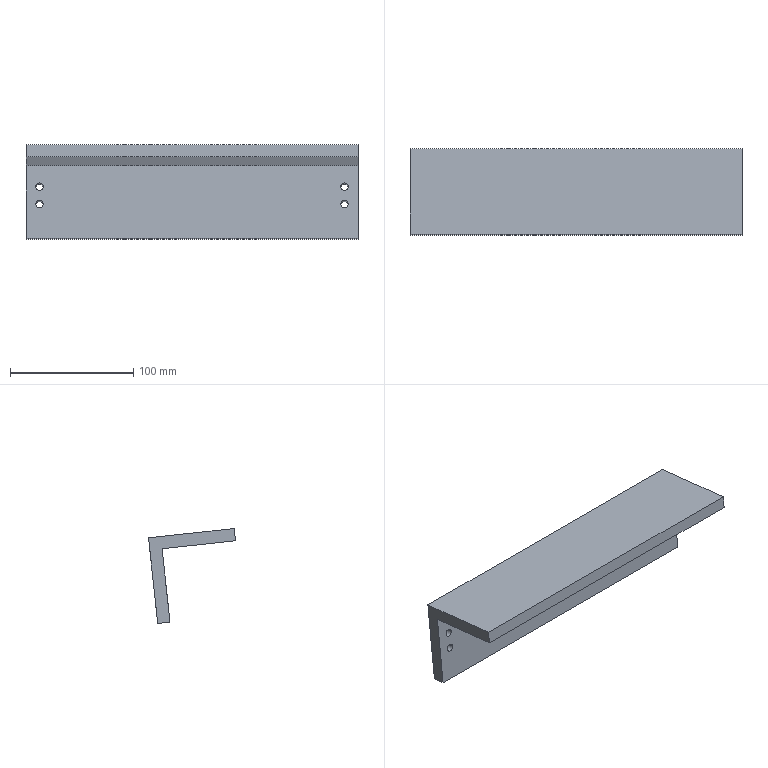Part | STEP file | Fillet 1-6 | 1 solid | 17 faces | box 269.706 x 70.669 x 77.109 mm | volume 349545 mm3 | cylinder 9 | plane 8 | commonest cylinder face diameters 6 x8 2 x1
STEP:
#1=CARTESIAN_POINT('',(40.034,-1255.734,3546.775));
#2=VERTEX_POINT('',#1);
#3=CARTESIAN_POINT('',(46.034,-1255.734,3546.775));
#4=VERTEX_POINT('',#3);
#5=CARTESIAN_POINT('',(43.034,-1255.734,3546.775));
#6=DIRECTION('',(0.,0.9942,-0.1073));
#7=DIRECTION('',(-1.,0.,0.));
#8=AXIS2_PLACEMENT_3D('',#5,#6,#7);
#9=CIRCLE('',#8,3.);
#10=EDGE_CURVE('',#2,#4,#9,.T.);
#11=ORIENTED_EDGE('',*,*,#10,.F.);
#12=CARTESIAN_POINT('',(40.034,-1245.792,3545.702));
#13=VERTEX_POINT('',#12);
#14=CARTESIAN_POINT('',(40.034,-1255.734,3546.775));
#15=DIRECTION('',(0.,0.9942,-0.1073));
#16=VECTOR('',#15,1000.);
#17=LINE('',#14,#16);
#18=EDGE_CURVE('',#2,#13,#17,.T.);
#19=ORIENTED_EDGE('',*,*,#18,.T.);
#20=CARTESIAN_POINT('',(46.034,-1245.792,3545.702));
#21=VERTEX_POINT('',#20);
#22=CARTESIAN_POINT('',(43.034,-1245.792,3545.702));
#23=DIRECTION('',(0.,0.9942,-0.1073));
#24=DIRECTION('',(-1.,0.,0.));
#25=AXIS2_PLACEMENT_3D('',#22,#23,#24);
#26=CIRCLE('',#25,3.);
#27=EDGE_CURVE('',#13,#21,#26,.T.);
#28=ORIENTED_EDGE('',*,*,#27,.T.);
#29=CARTESIAN_POINT('',(46.034,-1255.734,3546.775));
#30=DIRECTION('',(0.,0.9942,-0.1073));
#31=VECTOR('',#30,1000.);
#32=LINE('',#29,#31);
#33=EDGE_CURVE('',#4,#21,#32,.T.);
#34=ORIENTED_EDGE('',*,*,#33,.F.);
#35=EDGE_LOOP('',(#11,#19,#28,#34));
#36=FACE_OUTER_BOUND('',#35,.T.);
#37=CARTESIAN_POINT('',(43.034,-1255.734,3546.775));
#38=DIRECTION('',(0.,0.9942,-0.1073));
#39=DIRECTION('',(-1.,0.,0.));
#40=AXIS2_PLACEMENT_3D('',#37,#38,#39);
#41=CYLINDRICAL_SURFACE('',#40,3.);
#42=ADVANCED_FACE('',(#36),#41,.F.);
#43=CARTESIAN_POINT('',(287.74,-1254.205,3560.936));
#44=VERTEX_POINT('',#43);
#45=CARTESIAN_POINT('',(293.74,-1254.205,3560.936));
#46=VERTEX_POINT('',#45);
#47=CARTESIAN_POINT('',(290.74,-1254.205,3560.936));
#48=DIRECTION('',(0.,0.9942,-0.1073));
#49=DIRECTION('',(-1.,0.,0.));
#50=AXIS2_PLACEMENT_3D('',#47,#48,#49);
#51=CIRCLE('',#50,3.);
#52=EDGE_CURVE('',#44,#46,#51,.T.);
#53=ORIENTED_EDGE('',*,*,#52,.F.);
#54=CARTESIAN_POINT('',(287.74,-1244.263,3559.863));
#55=VERTEX_POINT('',#54);
#56=CARTESIAN_POINT('',(287.74,-1254.205,3560.936));
#57=DIRECTION('',(0.,0.9942,-0.1073));
#58=VECTOR('',#57,1000.);
#59=LINE('',#56,#58);
#60=EDGE_CURVE('',#44,#55,#59,.T.);
#61=ORIENTED_EDGE('',*,*,#60,.T.);
#62=CARTESIAN_POINT('',(293.74,-1244.263,3559.863));
#63=VERTEX_POINT('',#62);
#64=CARTESIAN_POINT('',(290.74,-1244.263,3559.863));
#65=DIRECTION('',(0.,0.9942,-0.1073));
#66=DIRECTION('',(-1.,0.,0.));
#67=AXIS2_PLACEMENT_3D('',#64,#65,#66);
#68=CIRCLE('',#67,3.);
#69=EDGE_CURVE('',#55,#63,#68,.T.);
#70=ORIENTED_EDGE('',*,*,#69,.T.);
#71=CARTESIAN_POINT('',(293.74,-1254.205,3560.936));
#72=DIRECTION('',(0.,0.9942,-0.1073));
#73=VECTOR('',#72,1000.);
#74=LINE('',#71,#73);
#75=EDGE_CURVE('',#46,#63,#74,.T.);
#76=ORIENTED_EDGE('',*,*,#75,.F.);
#77=EDGE_LOOP('',(#53,#61,#70,#76));
#78=FACE_OUTER_BOUND('',#77,.T.);
#79=CARTESIAN_POINT('',(290.74,-1254.205,3560.936));
#80=DIRECTION('',(0.,0.9942,-0.1073));
#81=DIRECTION('',(-1.,0.,0.));
#82=AXIS2_PLACEMENT_3D('',#79,#80,#81);
#83=CYLINDRICAL_SURFACE('',#82,3.);
#84=ADVANCED_FACE('',(#78),#83,.F.);
#85=CARTESIAN_POINT('',(287.74,-1255.734,3546.775));
#86=VERTEX_POINT('',#85);
#87=CARTESIAN_POINT('',(293.74,-1255.734,3546.775));
#88=VERTEX_POINT('',#87);
#89=CARTESIAN_POINT('',(290.74,-1255.734,3546.775));
#90=DIRECTION('',(0.,0.9942,-0.1073));
#91=DIRECTION('',(1.,0.,0.));
#92=AXIS2_PLACEMENT_3D('',#89,#90,#91);
#93=CIRCLE('',#92,3.);
#94=EDGE_CURVE('',#86,#88,#93,.T.);
#95=ORIENTED_EDGE('',*,*,#94,.F.);
#96=CARTESIAN_POINT('',(287.74,-1245.792,3545.702));
#97=VERTEX_POINT('',#96);
#98=CARTESIAN_POINT('',(287.74,-1255.734,3546.775));
#99=DIRECTION('',(0.,0.9942,-0.1073));
#100=VECTOR('',#99,1000.);
#101=LINE('',#98,#100);
#102=EDGE_CURVE('',#86,#97,#101,.T.);
#103=ORIENTED_EDGE('',*,*,#102,.T.);
#104=CARTESIAN_POINT('',(293.74,-1245.792,3545.702));
#105=VERTEX_POINT('',#104);
#106=CARTESIAN_POINT('',(290.74,-1245.792,3545.702));
#107=DIRECTION('',(0.,0.9942,-0.1073));
#108=DIRECTION('',(1.,0.,0.));
#109=AXIS2_PLACEMENT_3D('',#106,#107,#108);
#110=CIRCLE('',#109,3.);
#111=EDGE_CURVE('',#97,#105,#110,.T.);
#112=ORIENTED_EDGE('',*,*,#111,.T.);
#113=CARTESIAN_POINT('',(293.74,-1255.734,3546.775));
#114=DIRECTION('',(0.,0.9942,-0.1073));
#115=VECTOR('',#114,1000.);
#116=LINE('',#113,#115);
#117=EDGE_CURVE('',#88,#105,#116,.T.);
#118=ORIENTED_EDGE('',*,*,#117,.F.);
#119=EDGE_LOOP('',(#95,#103,#112,#118));
#120=FACE_OUTER_BOUND('',#119,.T.);
#121=CARTESIAN_POINT('',(290.74,-1255.734,3546.775));
#122=DIRECTION('',(0.,0.9942,-0.1073));
#123=DIRECTION('',(-1.,0.,0.));
#124=AXIS2_PLACEMENT_3D('',#121,#122,#123);
#125=CYLINDRICAL_SURFACE('',#124,3.);
#126=ADVANCED_FACE('',(#120),#125,.F.);
#127=CARTESIAN_POINT('',(40.034,-1254.205,3560.936));
#128=VERTEX_POINT('',#127);
#129=CARTESIAN_POINT('',(46.034,-1254.205,3560.936));
#130=VERTEX_POINT('',#129);
#131=CARTESIAN_POINT('',(43.034,-1254.205,3560.936));
#132=DIRECTION('',(0.,0.9942,-0.1073));
#133=DIRECTION('',(1.,0.,0.));
#134=AXIS2_PLACEMENT_3D('',#131,#132,#133);
#135=CIRCLE('',#134,3.);
#136=EDGE_CURVE('',#128,#130,#135,.T.);
#137=ORIENTED_EDGE('',*,*,#136,.F.);
#138=CARTESIAN_POINT('',(40.034,-1244.263,3559.863));
#139=VERTEX_POINT('',#138);
#140=CARTESIAN_POINT('',(40.034,-1254.205,3560.936));
#141=DIRECTION('',(0.,0.9942,-0.1073));
#142=VECTOR('',#141,1000.);
#143=LINE('',#140,#142);
#144=EDGE_CURVE('',#128,#139,#143,.T.);
#145=ORIENTED_EDGE('',*,*,#144,.T.);
#146=CARTESIAN_POINT('',(46.034,-1244.263,3559.863));
#147=VERTEX_POINT('',#146);
#148=CARTESIAN_POINT('',(43.034,-1244.263,3559.863));
#149=DIRECTION('',(0.,0.9942,-0.1073));
#150=DIRECTION('',(1.,0.,0.));
#151=AXIS2_PLACEMENT_3D('',#148,#149,#150);
#152=CIRCLE('',#151,3.);
#153=EDGE_CURVE('',#139,#147,#152,.T.);
#154=ORIENTED_EDGE('',*,*,#153,.T.);
#155=CARTESIAN_POINT('',(46.034,-1254.205,3560.936));
#156=DIRECTION('',(0.,0.9942,-0.1073));
#157=VECTOR('',#156,1000.);
#158=LINE('',#155,#157);
#159=EDGE_CURVE('',#130,#147,#158,.T.);
#160=ORIENTED_EDGE('',*,*,#159,.F.);
#161=EDGE_LOOP('',(#137,#145,#154,#160));
#162=FACE_OUTER_BOUND('',#161,.T.);
#163=CARTESIAN_POINT('',(43.034,-1254.205,3560.936));
#164=DIRECTION('',(0.,0.9942,-0.1073));
#165=DIRECTION('',(-1.,0.,0.));
#166=AXIS2_PLACEMENT_3D('',#163,#164,#165);
#167=CYLINDRICAL_SURFACE('',#166,3.);
#168=ADVANCED_FACE('',(#162),#167,.F.);
#169=CARTESIAN_POINT('',(43.034,-1255.734,3546.775));
#170=DIRECTION('',(0.,0.9942,-0.1073));
#171=DIRECTION('',(-1.,0.,0.));
#172=AXIS2_PLACEMENT_3D('',#169,#170,#171);
#173=CIRCLE('',#172,3.);
#174=EDGE_CURVE('',#4,#2,#173,.T.);
#175=ORIENTED_EDGE('',*,*,#174,.T.);
#176=ORIENTED_EDGE('',*,*,#10,.T.);
#177=EDGE_LOOP('',(#175,#176));
#178=FACE_BOUND('',#177,.T.);
#179=CARTESIAN_POINT('',(290.74,-1254.205,3560.936));
#180=DIRECTION('',(0.,0.9942,-0.1073));
#181=DIRECTION('',(-1.,0.,0.));
#182=AXIS2_PLACEMENT_3D('',#179,#180,#181);
#183=CIRCLE('',#182,3.);
#184=EDGE_CURVE('',#46,#44,#183,.T.);
#185=ORIENTED_EDGE('',*,*,#184,.T.);
#186=ORIENTED_EDGE('',*,*,#52,.T.);
#187=EDGE_LOOP('',(#185,#186));
#188=FACE_BOUND('',#187,.T.);
#189=CARTESIAN_POINT('',(290.74,-1255.734,3546.775));
#190=DIRECTION('',(0.,0.9942,-0.1073));
#191=DIRECTION('',(1.,0.,0.));
#192=AXIS2_PLACEMENT_3D('',#189,#190,#191);
#193=CIRCLE('',#192,3.);
#194=EDGE_CURVE('',#88,#86,#193,.T.);
#195=ORIENTED_EDGE('',*,*,#194,.T.);
#196=ORIENTED_EDGE('',*,*,#94,.T.);
#197=EDGE_LOOP('',(#195,#196));
#198=FACE_BOUND('',#197,.T.);
#199=CARTESIAN_POINT('',(43.034,-1254.205,3560.936));
#200=DIRECTION('',(0.,0.9942,-0.1073));
#201=DIRECTION('',(1.,0.,0.));
#202=AXIS2_PLACEMENT_3D('',#199,#200,#201);
#203=CIRCLE('',#202,3.);
#204=EDGE_CURVE('',#130,#128,#203,.T.);
#205=ORIENTED_EDGE('',*,*,#204,.T.);
#206=ORIENTED_EDGE('',*,*,#136,.T.);
#207=EDGE_LOOP('',(#205,#206));
#208=FACE_BOUND('',#207,.T.);
#209=CARTESIAN_POINT('',(301.74,-1252.394,3577.717));
#210=VERTEX_POINT('',#209);
#211=CARTESIAN_POINT('',(301.74,-1258.727,3519.058));
#212=VERTEX_POINT('',#211);
#213=CARTESIAN_POINT('',(301.74,-1251.213,3588.654));
#214=DIRECTION('',(0.,-0.1073,-0.9942));
#215=VECTOR('',#214,1000.);
#216=LINE('',#213,#215);
#217=EDGE_CURVE('',#210,#212,#216,.T.);
#218=ORIENTED_EDGE('',*,*,#217,.F.);
#219=CARTESIAN_POINT('',(32.034,-1252.394,3577.717));
#220=VERTEX_POINT('',#219);
#221=CARTESIAN_POINT('',(166.887,-1252.394,3577.717));
#222=DIRECTION('',(-1.,0.,0.));
#223=VECTOR('',#222,1000.);
#224=LINE('',#221,#223);
#225=EDGE_CURVE('',#210,#220,#224,.T.);
#226=ORIENTED_EDGE('',*,*,#225,.T.);
#227=CARTESIAN_POINT('',(32.034,-1258.727,3519.058));
#228=VERTEX_POINT('',#227);
#229=CARTESIAN_POINT('',(32.034,-1251.213,3588.654));
#230=DIRECTION('',(0.,0.1073,0.9942));
#231=VECTOR('',#230,1000.);
#232=LINE('',#229,#231);
#233=EDGE_CURVE('',#228,#220,#232,.T.);
#234=ORIENTED_EDGE('',*,*,#233,.F.);
#235=CARTESIAN_POINT('',(32.034,-1258.727,3519.058));
#236=DIRECTION('',(-1.,0.,0.));
#237=VECTOR('',#236,1000.);
#238=LINE('',#235,#237);
#239=EDGE_CURVE('',#212,#228,#238,.T.);
#240=ORIENTED_EDGE('',*,*,#239,.F.);
#241=EDGE_LOOP('',(#218,#226,#234,#240));
#242=FACE_OUTER_BOUND('',#241,.T.);
#243=CARTESIAN_POINT('',(166.887,-1254.97,3553.856));
#244=DIRECTION('',(0.,-0.9942,0.1073));
#245=DIRECTION('',(1.,0.,0.));
#246=AXIS2_PLACEMENT_3D('',#243,#244,#245);
#247=PLANE('',#246);
#248=ADVANCED_FACE('',(#178,#188,#198,#208,#242),#247,.T.);
#249=CARTESIAN_POINT('',(301.74,-1241.271,3587.58));
#250=VERTEX_POINT('',#249);
#251=CARTESIAN_POINT('',(301.74,-1310.866,3595.094));
#252=VERTEX_POINT('',#251);
#253=CARTESIAN_POINT('',(301.74,-1241.271,3587.58));
#254=DIRECTION('',(0.,-0.9942,0.1073));
#255=VECTOR('',#254,1000.);
#256=LINE('',#253,#255);
#257=EDGE_CURVE('',#250,#252,#256,.T.);
#258=ORIENTED_EDGE('',*,*,#257,.T.);
#259=CARTESIAN_POINT('',(301.74,-1311.94,3585.152));
#260=VERTEX_POINT('',#259);
#261=CARTESIAN_POINT('',(301.74,-1311.94,3585.152));
#262=DIRECTION('',(0.,0.1073,0.9942));
#263=VECTOR('',#262,1000.);
#264=LINE('',#261,#263);
#265=EDGE_CURVE('',#260,#252,#264,.T.);
#266=ORIENTED_EDGE('',*,*,#265,.F.);
#267=CARTESIAN_POINT('',(301.74,-1253.281,3578.819));
#268=VERTEX_POINT('',#267);
#269=CARTESIAN_POINT('',(301.74,-1311.94,3585.152));
#270=DIRECTION('',(0.,0.9942,-0.1073));
#271=VECTOR('',#270,1000.);
#272=LINE('',#269,#271);
#273=EDGE_CURVE('',#260,#268,#272,.T.);
#274=ORIENTED_EDGE('',*,*,#273,.T.);
#275=CARTESIAN_POINT('',(301.74,-1253.388,3577.825));
#276=DIRECTION('',(-1.,0.,0.));
#277=DIRECTION('',(0.,0.9942,-0.1073));
#278=AXIS2_PLACEMENT_3D('',#275,#276,#277);
#279=CIRCLE('',#278,1.);
#280=EDGE_CURVE('',#268,#210,#279,.T.);
#281=ORIENTED_EDGE('',*,*,#280,.T.);
#282=ORIENTED_EDGE('',*,*,#217,.T.);
#283=CARTESIAN_POINT('',(301.74,-1248.785,3517.985));
#284=VERTEX_POINT('',#283);
#285=CARTESIAN_POINT('',(301.74,-1248.785,3517.985));
#286=DIRECTION('',(0.,-0.9942,0.1073));
#287=VECTOR('',#286,1000.);
#288=LINE('',#285,#287);
#289=EDGE_CURVE('',#284,#212,#288,.T.);
#290=ORIENTED_EDGE('',*,*,#289,.F.);
#291=CARTESIAN_POINT('',(301.74,-1241.271,3587.58));
#292=DIRECTION('',(0.,-0.1073,-0.9942));
#293=VECTOR('',#292,1000.);
#294=LINE('',#291,#293);
#295=EDGE_CURVE('',#250,#284,#294,.T.);
#296=ORIENTED_EDGE('',*,*,#295,.F.);
#297=EDGE_LOOP('',(#258,#266,#274,#281,#282,#290,#296));
#298=FACE_OUTER_BOUND('',#297,.T.);
#299=CARTESIAN_POINT('',(301.74,-1241.271,3587.58));
#300=DIRECTION('',(-1.,0.,0.));
#301=DIRECTION('',(0.,-0.9942,0.1073));
#302=AXIS2_PLACEMENT_3D('',#299,#300,#301);
#303=PLANE('',#302);
#304=ADVANCED_FACE('',(#298),#303,.F.);
#305=ORIENTED_EDGE('',*,*,#239,.T.);
#306=CARTESIAN_POINT('',(32.034,-1248.785,3517.985));
#307=VERTEX_POINT('',#306);
#308=CARTESIAN_POINT('',(32.034,-1248.785,3517.985));
#309=DIRECTION('',(0.,-0.9942,0.1073));
#310=VECTOR('',#309,1000.);
#311=LINE('',#308,#310);
#312=EDGE_CURVE('',#307,#228,#311,.T.);
#313=ORIENTED_EDGE('',*,*,#312,.F.);
#314=CARTESIAN_POINT('',(32.034,-1248.785,3517.985));
#315=DIRECTION('',(-1.,0.,0.));
#316=VECTOR('',#315,1000.);
#317=LINE('',#314,#316);
#318=EDGE_CURVE('',#284,#307,#317,.T.);
#319=ORIENTED_EDGE('',*,*,#318,.F.);
#320=ORIENTED_EDGE('',*,*,#289,.T.);
#321=EDGE_LOOP('',(#305,#313,#319,#320));
#322=FACE_OUTER_BOUND('',#321,.T.);
#323=CARTESIAN_POINT('',(32.034,-1248.785,3517.985));
#324=DIRECTION('',(0.,0.1073,0.9942));
#325=DIRECTION('',(0.,0.9942,-0.1073));
#326=AXIS2_PLACEMENT_3D('',#323,#324,#325);
#327=PLANE('',#326);
#328=ADVANCED_FACE('',(#322),#327,.F.);
#329=ORIENTED_EDGE('',*,*,#233,.T.);
#330=CARTESIAN_POINT('',(32.034,-1253.281,3578.819));
#331=VERTEX_POINT('',#330);
#332=CARTESIAN_POINT('',(32.034,-1253.388,3577.825));
#333=DIRECTION('',(1.,0.,0.));
#334=DIRECTION('',(0.,-0.9942,0.1073));
#335=AXIS2_PLACEMENT_3D('',#332,#333,#334);
#336=CIRCLE('',#335,1.);
#337=EDGE_CURVE('',#220,#331,#336,.T.);
#338=ORIENTED_EDGE('',*,*,#337,.T.);
#339=CARTESIAN_POINT('',(32.034,-1311.94,3585.152));
#340=VERTEX_POINT('',#339);
#341=CARTESIAN_POINT('',(32.034,-1252.286,3578.711));
#342=DIRECTION('',(0.,-0.9942,0.1073));
#343=VECTOR('',#342,1000.);
#344=LINE('',#341,#343);
#345=EDGE_CURVE('',#331,#340,#344,.T.);
#346=ORIENTED_EDGE('',*,*,#345,.T.);
#347=CARTESIAN_POINT('',(32.034,-1310.866,3595.094));
#348=VERTEX_POINT('',#347);
#349=CARTESIAN_POINT('',(32.034,-1311.94,3585.152));
#350=DIRECTION('',(0.,0.1073,0.9942));
#351=VECTOR('',#350,1000.);
#352=LINE('',#349,#351);
#353=EDGE_CURVE('',#340,#348,#352,.T.);
#354=ORIENTED_EDGE('',*,*,#353,.T.);
#355=CARTESIAN_POINT('',(32.034,-1241.271,3587.58));
#356=VERTEX_POINT('',#355);
#357=CARTESIAN_POINT('',(32.034,-1241.271,3587.58));
#358=DIRECTION('',(0.,-0.9942,0.1073));
#359=VECTOR('',#358,1000.);
#360=LINE('',#357,#359);
#361=EDGE_CURVE('',#356,#348,#360,.T.);
#362=ORIENTED_EDGE('',*,*,#361,.F.);
#363=CARTESIAN_POINT('',(32.034,-1241.271,3587.58));
#364=DIRECTION('',(0.,0.1073,0.9942));
#365=VECTOR('',#364,1000.);
#366=LINE('',#363,#365);
#367=EDGE_CURVE('',#307,#356,#366,.T.);
#368=ORIENTED_EDGE('',*,*,#367,.F.);
#369=ORIENTED_EDGE('',*,*,#312,.T.);
#370=EDGE_LOOP('',(#329,#338,#346,#354,#362,#368,#369));
#371=FACE_OUTER_BOUND('',#370,.T.);
#372=CARTESIAN_POINT('',(32.034,-1241.271,3587.58));
#373=DIRECTION('',(1.,0.,0.));
#374=DIRECTION('',(0.,0.9942,-0.1073));
#375=AXIS2_PLACEMENT_3D('',#372,#373,#374);
#376=PLANE('',#375);
#377=ADVANCED_FACE('',(#371),#376,.F.);
#378=ORIENTED_EDGE('',*,*,#361,.T.);
#379=CARTESIAN_POINT('',(32.034,-1310.866,3595.094));
#380=DIRECTION('',(1.,0.,0.));
#381=VECTOR('',#380,1000.);
#382=LINE('',#379,#381);
#383=EDGE_CURVE('',#348,#252,#382,.T.);
#384=ORIENTED_EDGE('',*,*,#383,.T.);
#385=ORIENTED_EDGE('',*,*,#257,.F.);
#386=CARTESIAN_POINT('',(32.034,-1241.271,3587.58));
#387=DIRECTION('',(1.,0.,0.));
#388=VECTOR('',#387,1000.);
#389=LINE('',#386,#388);
#390=EDGE_CURVE('',#356,#250,#389,.T.);
#391=ORIENTED_EDGE('',*,*,#390,.F.);
#392=EDGE_LOOP('',(#378,#384,#385,#391));
#393=FACE_OUTER_BOUND('',#392,.T.);
#394=CARTESIAN_POINT('',(32.034,-1241.271,3587.58));
#395=DIRECTION('',(0.,-0.1073,-0.9942));
#396=DIRECTION('',(0.,-0.9942,0.1073));
#397=AXIS2_PLACEMENT_3D('',#394,#395,#396);
#398=PLANE('',#397);
#399=ADVANCED_FACE('',(#393),#398,.F.);
#400=CARTESIAN_POINT('',(43.034,-1245.792,3545.702));
#401=DIRECTION('',(0.,0.9942,-0.1073));
#402=DIRECTION('',(-1.,0.,0.));
#403=AXIS2_PLACEMENT_3D('',#400,#401,#402);
#404=CIRCLE('',#403,3.);
#405=EDGE_CURVE('',#21,#13,#404,.T.);
#406=ORIENTED_EDGE('',*,*,#405,.F.);
#407=ORIENTED_EDGE('',*,*,#27,.F.);
#408=EDGE_LOOP('',(#406,#407));
#409=FACE_BOUND('',#408,.T.);
#410=CARTESIAN_POINT('',(290.74,-1244.263,3559.863));
#411=DIRECTION('',(0.,0.9942,-0.1073));
#412=DIRECTION('',(-1.,0.,0.));
#413=AXIS2_PLACEMENT_3D('',#410,#411,#412);
#414=CIRCLE('',#413,3.);
#415=EDGE_CURVE('',#63,#55,#414,.T.);
#416=ORIENTED_EDGE('',*,*,#415,.F.);
#417=ORIENTED_EDGE('',*,*,#69,.F.);
#418=EDGE_LOOP('',(#416,#417));
#419=FACE_BOUND('',#418,.T.);
#420=CARTESIAN_POINT('',(290.74,-1245.792,3545.702));
#421=DIRECTION('',(0.,0.9942,-0.1073));
#422=DIRECTION('',(1.,0.,0.));
#423=AXIS2_PLACEMENT_3D('',#420,#421,#422);
#424=CIRCLE('',#423,3.);
#425=EDGE_CURVE('',#105,#97,#424,.T.);
#426=ORIENTED_EDGE('',*,*,#425,.F.);
#427=ORIENTED_EDGE('',*,*,#111,.F.);
#428=EDGE_LOOP('',(#426,#427));
#429=FACE_BOUND('',#428,.T.);
#430=CARTESIAN_POINT('',(43.034,-1244.263,3559.863));
#431=DIRECTION('',(0.,0.9942,-0.1073));
#432=DIRECTION('',(1.,0.,0.));
#433=AXIS2_PLACEMENT_3D('',#430,#431,#432);
#434=CIRCLE('',#433,3.);
#435=EDGE_CURVE('',#147,#139,#434,.T.);
#436=ORIENTED_EDGE('',*,*,#435,.F.);
#437=ORIENTED_EDGE('',*,*,#153,.F.);
#438=EDGE_LOOP('',(#436,#437));
#439=FACE_BOUND('',#438,.T.);
#440=ORIENTED_EDGE('',*,*,#295,.T.);
#441=ORIENTED_EDGE('',*,*,#318,.T.);
#442=ORIENTED_EDGE('',*,*,#367,.T.);
#443=ORIENTED_EDGE('',*,*,#390,.T.);
#444=EDGE_LOOP('',(#440,#441,#442,#443));
#445=FACE_OUTER_BOUND('',#444,.T.);
#446=CARTESIAN_POINT('',(166.887,-1245.028,3552.782));
#447=DIRECTION('',(0.,-0.9942,0.1073));
#448=DIRECTION('',(1.,0.,0.));
#449=AXIS2_PLACEMENT_3D('',#446,#447,#448);
#450=PLANE('',#449);
#451=ADVANCED_FACE('',(#409,#419,#429,#439,#445),#450,.F.);
#452=ORIENTED_EDGE('',*,*,#144,.F.);
#453=ORIENTED_EDGE('',*,*,#204,.F.);
#454=ORIENTED_EDGE('',*,*,#159,.T.);
#455=ORIENTED_EDGE('',*,*,#435,.T.);
#456=EDGE_LOOP('',(#452,#453,#454,#455));
#457=FACE_OUTER_BOUND('',#456,.T.);
#458=CARTESIAN_POINT('',(43.034,-1254.205,3560.936));
#459=DIRECTION('',(0.,0.9942,-0.1073));
#460=DIRECTION('',(-1.,0.,0.));
#461=AXIS2_PLACEMENT_3D('',#458,#459,#460);
#462=CYLINDRICAL_SURFACE('',#461,3.);
#463=ADVANCED_FACE('',(#457),#462,.F.);
#464=ORIENTED_EDGE('',*,*,#102,.F.);
#465=ORIENTED_EDGE('',*,*,#194,.F.);
#466=ORIENTED_EDGE('',*,*,#117,.T.);
#467=ORIENTED_EDGE('',*,*,#425,.T.);
#468=EDGE_LOOP('',(#464,#465,#466,#467));
#469=FACE_OUTER_BOUND('',#468,.T.);
#470=CARTESIAN_POINT('',(290.74,-1255.734,3546.775));
#471=DIRECTION('',(0.,0.9942,-0.1073));
#472=DIRECTION('',(-1.,0.,0.));
#473=AXIS2_PLACEMENT_3D('',#470,#471,#472);
#474=CYLINDRICAL_SURFACE('',#473,3.);
#475=ADVANCED_FACE('',(#469),#474,.F.);
#476=ORIENTED_EDGE('',*,*,#60,.F.);
#477=ORIENTED_EDGE('',*,*,#184,.F.);
#478=ORIENTED_EDGE('',*,*,#75,.T.);
#479=ORIENTED_EDGE('',*,*,#415,.T.);
#480=EDGE_LOOP('',(#476,#477,#478,#479));
#481=FACE_OUTER_BOUND('',#480,.T.);
#482=CARTESIAN_POINT('',(290.74,-1254.205,3560.936));
#483=DIRECTION('',(0.,0.9942,-0.1073));
#484=DIRECTION('',(-1.,0.,0.));
#485=AXIS2_PLACEMENT_3D('',#482,#483,#484);
#486=CYLINDRICAL_SURFACE('',#485,3.);
#487=ADVANCED_FACE('',(#481),#486,.F.);
#488=ORIENTED_EDGE('',*,*,#18,.F.);
#489=ORIENTED_EDGE('',*,*,#174,.F.);
#490=ORIENTED_EDGE('',*,*,#33,.T.);
#491=ORIENTED_EDGE('',*,*,#405,.T.);
#492=EDGE_LOOP('',(#488,#489,#490,#491));
#493=FACE_OUTER_BOUND('',#492,.T.);
#494=CARTESIAN_POINT('',(43.034,-1255.734,3546.775));
#495=DIRECTION('',(0.,0.9942,-0.1073));
#496=DIRECTION('',(-1.,0.,0.));
#497=AXIS2_PLACEMENT_3D('',#494,#495,#496);
#498=CYLINDRICAL_SURFACE('',#497,3.);
#499=ADVANCED_FACE('',(#493),#498,.F.);
#500=ORIENTED_EDGE('',*,*,#383,.F.);
#501=ORIENTED_EDGE('',*,*,#353,.F.);
#502=CARTESIAN_POINT('',(32.034,-1311.94,3585.152));
#503=DIRECTION('',(1.,0.,0.));
#504=VECTOR('',#503,1000.);
#505=LINE('',#502,#504);
#506=EDGE_CURVE('',#340,#260,#505,.T.);
#507=ORIENTED_EDGE('',*,*,#506,.T.);
#508=ORIENTED_EDGE('',*,*,#265,.T.);
#509=EDGE_LOOP('',(#500,#501,#507,#508));
#510=FACE_OUTER_BOUND('',#509,.T.);
#511=CARTESIAN_POINT('',(32.034,-1311.94,3585.152));
#512=DIRECTION('',(0.,-0.9942,0.1073));
#513=DIRECTION('',(1.,0.,0.));
#514=AXIS2_PLACEMENT_3D('',#511,#512,#513);
#515=PLANE('',#514);
#516=ADVANCED_FACE('',(#510),#515,.T.);
#517=ORIENTED_EDGE('',*,*,#345,.F.);
#518=CARTESIAN_POINT('',(166.887,-1253.281,3578.819));
#519=DIRECTION('',(1.,0.,0.));
#520=VECTOR('',#519,1000.);
#521=LINE('',#518,#520);
#522=EDGE_CURVE('',#331,#268,#521,.T.);
#523=ORIENTED_EDGE('',*,*,#522,.T.);
#524=ORIENTED_EDGE('',*,*,#273,.F.);
#525=ORIENTED_EDGE('',*,*,#506,.F.);
#526=EDGE_LOOP('',(#517,#523,#524,#525));
#527=FACE_OUTER_BOUND('',#526,.T.);
#528=CARTESIAN_POINT('',(166.887,-1252.286,3578.711));
#529=DIRECTION('',(0.,0.1073,0.9942));
#530=DIRECTION('',(0.,0.9942,-0.1073));
#531=AXIS2_PLACEMENT_3D('',#528,#529,#530);
#532=PLANE('',#531);
#533=ADVANCED_FACE('',(#527),#532,.F.);
#534=ORIENTED_EDGE('',*,*,#280,.F.);
#535=ORIENTED_EDGE('',*,*,#522,.F.);
#536=ORIENTED_EDGE('',*,*,#337,.F.);
#537=ORIENTED_EDGE('',*,*,#225,.F.);
#538=EDGE_LOOP('',(#534,#535,#536,#537));
#539=FACE_OUTER_BOUND('',#538,.T.);
#540=CARTESIAN_POINT('',(166.887,-1253.388,3577.825));
#541=DIRECTION('',(-1.,0.,0.));
#542=DIRECTION('',(0.,-0.9942,0.1073));
#543=AXIS2_PLACEMENT_3D('',#540,#541,#542);
#544=CYLINDRICAL_SURFACE('',#543,1.);
#545=ADVANCED_FACE('',(#539),#544,.F.);
#546=CLOSED_SHELL('',(#42,#84,#126,#168,#248,#304,#328,#377,#399,#451,#463,#475,#487,#499,#516,#533,#545));
#547=MANIFOLD_SOLID_BREP('',#546);
#548=CARTESIAN_POINT('',(0.,0.,0.));
#549=DIRECTION('',(0.,0.,1.));
#550=DIRECTION('',(1.,0.,0.));
#551=AXIS2_PLACEMENT_3D('',#548,#549,#550);
#552=(LENGTH_UNIT()NAMED_UNIT(*)SI_UNIT(.MILLI.,.METRE.));
#553=UNCERTAINTY_MEASURE_WITH_UNIT(LENGTH_MEASURE(0.00001),#552,'','');
#554=(NAMED_UNIT(*)PLANE_ANGLE_UNIT()SI_UNIT($,.RADIAN.));
#555=(NAMED_UNIT(*)SI_UNIT($,.STERADIAN.)SOLID_ANGLE_UNIT());
#556=(GEOMETRIC_REPRESENTATION_CONTEXT(3)GLOBAL_UNCERTAINTY_ASSIGNED_CONTEXT((#553))GLOBAL_UNIT_ASSIGNED_CONTEXT((#552,#554,#555))REPRESENTATION_CONTEXT('',''));
#557=ADVANCED_BREP_SHAPE_REPRESENTATION('',(#547,#551),#556);